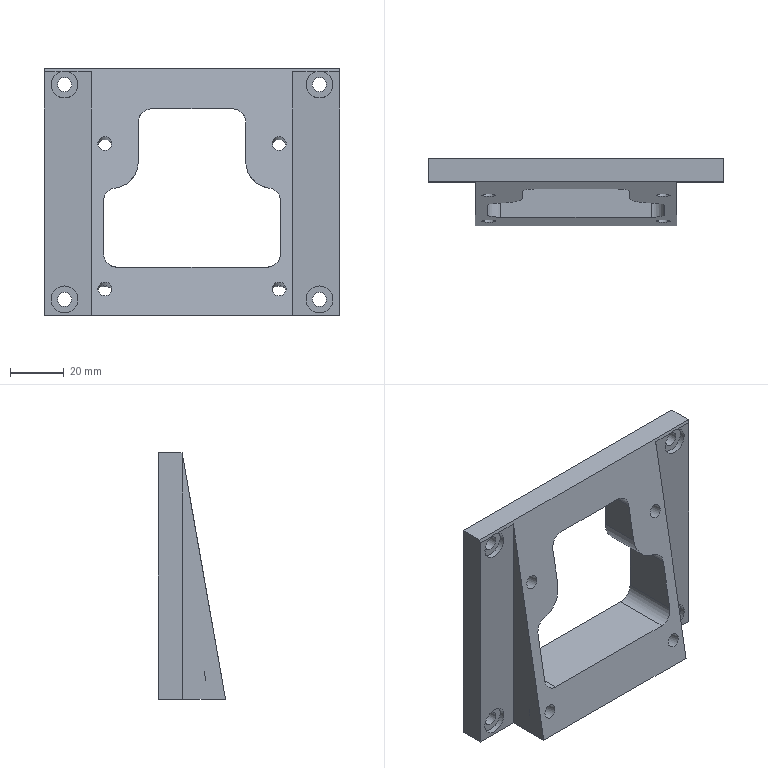Part | 1 solid | 48 faces | box 110 x 25 x 92 mm | volume 85640 mm3 | plane 24 | cylinder 24 | commonest cylinder face diameters 10 x14 5.2 x4 5.3 x4 20 x2
STEP:
#1=CARTESIAN_POINT('',(-37.5,3.5,44.741));
#2=VERTEX_POINT('',#1);
#3=CARTESIAN_POINT('',(-37.5,-12.5,-46.));
#4=VERTEX_POINT('',#3);
#5=CARTESIAN_POINT('',(-37.5,3.5,44.741));
#6=DIRECTION('',(0.,-0.1736,-0.9848));
#7=VECTOR('',#6,1000.);
#8=LINE('',#5,#7);
#9=EDGE_CURVE('',#2,#4,#8,.T.);
#10=ORIENTED_EDGE('',*,*,#9,.F.);
#11=CARTESIAN_POINT('',(-37.5,3.5,-46.));
#12=VERTEX_POINT('',#11);
#13=CARTESIAN_POINT('',(-37.5,3.5,-46.));
#14=DIRECTION('',(0.,0.,1.));
#15=VECTOR('',#14,1000.);
#16=LINE('',#13,#15);
#17=EDGE_CURVE('',#12,#2,#16,.T.);
#18=ORIENTED_EDGE('',*,*,#17,.F.);
#19=CARTESIAN_POINT('',(-37.5,-12.5,-46.));
#20=DIRECTION('',(0.,1.,0.));
#21=VECTOR('',#20,1000.);
#22=LINE('',#19,#21);
#23=EDGE_CURVE('',#4,#12,#22,.T.);
#24=ORIENTED_EDGE('',*,*,#23,.F.);
#25=EDGE_LOOP('',(#10,#18,#24));
#26=FACE_BOUND('',#25,.T.);
#27=CARTESIAN_POINT('',(-37.5,3.5,-46.));
#28=DIRECTION('',(1.,0.,0.));
#29=DIRECTION('',(0.,-1.,0.));
#30=AXIS2_PLACEMENT_3D('',#27,#28,#29);
#31=PLANE('',#30);
#32=ADVANCED_FACE('',(#26),#31,.F.);
#33=CARTESIAN_POINT('',(50.15,12.5,-40.));
#34=VERTEX_POINT('',#33);
#35=CARTESIAN_POINT('',(47.5,12.5,-40.));
#36=DIRECTION('',(0.,-1.,0.));
#37=DIRECTION('',(1.,0.,0.));
#38=AXIS2_PLACEMENT_3D('',#35,#36,#37);
#39=CIRCLE('',#38,2.65);
#40=EDGE_CURVE('',#34,#34,#39,.T.);
#41=ORIENTED_EDGE('',*,*,#40,.F.);
#42=EDGE_LOOP('',(#41));
#43=FACE_BOUND('',#42,.T.);
#44=CARTESIAN_POINT('',(44.85,5.5,-40.));
#45=VERTEX_POINT('',#44);
#46=CARTESIAN_POINT('',(47.5,5.5,-40.));
#47=DIRECTION('',(0.,1.,0.));
#48=DIRECTION('',(-1.,0.,0.));
#49=AXIS2_PLACEMENT_3D('',#46,#47,#48);
#50=CIRCLE('',#49,2.65);
#51=EDGE_CURVE('',#45,#45,#50,.T.);
#52=ORIENTED_EDGE('',*,*,#51,.F.);
#53=EDGE_LOOP('',(#52));
#54=FACE_BOUND('',#53,.T.);
#55=CARTESIAN_POINT('',(47.5,-16.47,-40.));
#56=DIRECTION('',(0.,-1.,0.));
#57=DIRECTION('',(-1.,0.,0.));
#58=AXIS2_PLACEMENT_3D('',#55,#56,#57);
#59=CYLINDRICAL_SURFACE('',#58,2.65);
#60=ADVANCED_FACE('',(#43,#54),#59,.F.);
#61=CARTESIAN_POINT('',(50.15,12.5,40.));
#62=VERTEX_POINT('',#61);
#63=CARTESIAN_POINT('',(47.5,12.5,40.));
#64=DIRECTION('',(0.,-1.,0.));
#65=DIRECTION('',(1.,0.,0.));
#66=AXIS2_PLACEMENT_3D('',#63,#64,#65);
#67=CIRCLE('',#66,2.65);
#68=EDGE_CURVE('',#62,#62,#67,.T.);
#69=ORIENTED_EDGE('',*,*,#68,.F.);
#70=EDGE_LOOP('',(#69));
#71=FACE_BOUND('',#70,.T.);
#72=CARTESIAN_POINT('',(44.85,5.5,40.));
#73=VERTEX_POINT('',#72);
#74=CARTESIAN_POINT('',(47.5,5.5,40.));
#75=DIRECTION('',(0.,1.,0.));
#76=DIRECTION('',(-1.,0.,0.));
#77=AXIS2_PLACEMENT_3D('',#74,#75,#76);
#78=CIRCLE('',#77,2.65);
#79=EDGE_CURVE('',#73,#73,#78,.T.);
#80=ORIENTED_EDGE('',*,*,#79,.F.);
#81=EDGE_LOOP('',(#80));
#82=FACE_BOUND('',#81,.T.);
#83=CARTESIAN_POINT('',(47.5,-16.47,40.));
#84=DIRECTION('',(0.,-1.,0.));
#85=DIRECTION('',(-1.,0.,0.));
#86=AXIS2_PLACEMENT_3D('',#83,#84,#85);
#87=CYLINDRICAL_SURFACE('',#86,2.65);
#88=ADVANCED_FACE('',(#71,#82),#87,.F.);
#89=CARTESIAN_POINT('',(-50.15,12.5,-40.));
#90=VERTEX_POINT('',#89);
#91=CARTESIAN_POINT('',(-47.5,12.5,-40.));
#92=DIRECTION('',(0.,1.,0.));
#93=DIRECTION('',(-1.,0.,0.));
#94=AXIS2_PLACEMENT_3D('',#91,#92,#93);
#95=CIRCLE('',#94,2.65);
#96=EDGE_CURVE('',#90,#90,#95,.T.);
#97=ORIENTED_EDGE('',*,*,#96,.T.);
#98=EDGE_LOOP('',(#97));
#99=FACE_BOUND('',#98,.T.);
#100=CARTESIAN_POINT('',(-44.85,5.5,-40.));
#101=VERTEX_POINT('',#100);
#102=CARTESIAN_POINT('',(-47.5,5.5,-40.));
#103=DIRECTION('',(0.,-1.,0.));
#104=DIRECTION('',(1.,0.,0.));
#105=AXIS2_PLACEMENT_3D('',#102,#103,#104);
#106=CIRCLE('',#105,2.65);
#107=EDGE_CURVE('',#101,#101,#106,.T.);
#108=ORIENTED_EDGE('',*,*,#107,.T.);
#109=EDGE_LOOP('',(#108));
#110=FACE_BOUND('',#109,.T.);
#111=CARTESIAN_POINT('',(-47.5,-16.47,-40.));
#112=DIRECTION('',(0.,1.,0.));
#113=DIRECTION('',(1.,0.,0.));
#114=AXIS2_PLACEMENT_3D('',#111,#112,#113);
#115=CYLINDRICAL_SURFACE('',#114,2.65);
#116=ADVANCED_FACE('',(#99,#110),#115,.F.);
#117=CARTESIAN_POINT('',(-50.15,12.5,40.));
#118=VERTEX_POINT('',#117);
#119=CARTESIAN_POINT('',(-47.5,12.5,40.));
#120=DIRECTION('',(0.,1.,0.));
#121=DIRECTION('',(-1.,0.,0.));
#122=AXIS2_PLACEMENT_3D('',#119,#120,#121);
#123=CIRCLE('',#122,2.65);
#124=EDGE_CURVE('',#118,#118,#123,.T.);
#125=ORIENTED_EDGE('',*,*,#124,.T.);
#126=EDGE_LOOP('',(#125));
#127=FACE_BOUND('',#126,.T.);
#128=CARTESIAN_POINT('',(-44.85,5.5,40.));
#129=VERTEX_POINT('',#128);
#130=CARTESIAN_POINT('',(-47.5,5.5,40.));
#131=DIRECTION('',(0.,-1.,0.));
#132=DIRECTION('',(1.,0.,0.));
#133=AXIS2_PLACEMENT_3D('',#130,#131,#132);
#134=CIRCLE('',#133,2.65);
#135=EDGE_CURVE('',#129,#129,#134,.T.);
#136=ORIENTED_EDGE('',*,*,#135,.T.);
#137=EDGE_LOOP('',(#136));
#138=FACE_BOUND('',#137,.T.);
#139=CARTESIAN_POINT('',(-47.5,-16.452,40.));
#140=DIRECTION('',(0.,1.,0.));
#141=DIRECTION('',(1.,0.,0.));
#142=AXIS2_PLACEMENT_3D('',#139,#140,#141);
#143=CYLINDRICAL_SURFACE('',#142,2.65);
#144=ADVANCED_FACE('',(#127,#138),#143,.F.);
#145=CARTESIAN_POINT('',(-47.5,5.5,45.));
#146=VERTEX_POINT('',#145);
#147=CARTESIAN_POINT('',(-47.5,5.5,40.));
#148=DIRECTION('',(0.,-1.,0.));
#149=DIRECTION('',(0.,0.,1.));
#150=AXIS2_PLACEMENT_3D('',#147,#148,#149);
#151=CIRCLE('',#150,5.);
#152=EDGE_CURVE('',#146,#146,#151,.T.);
#153=ORIENTED_EDGE('',*,*,#152,.F.);
#154=EDGE_LOOP('',(#153));
#155=FACE_BOUND('',#154,.T.);
#156=CARTESIAN_POINT('',(-45.91,3.5,44.741));
#157=VERTEX_POINT('',#156);
#158=CARTESIAN_POINT('',(-49.09,3.5,44.741));
#159=VERTEX_POINT('',#158);
#160=CARTESIAN_POINT('',(-47.5,3.5,40.));
#161=DIRECTION('',(0.,1.,0.));
#162=DIRECTION('',(0.318,0.,0.9481));
#163=AXIS2_PLACEMENT_3D('',#160,#161,#162);
#164=CIRCLE('',#163,5.);
#165=EDGE_CURVE('',#157,#159,#164,.T.);
#166=ORIENTED_EDGE('',*,*,#165,.F.);
#167=CARTESIAN_POINT('',(-47.5,2.664,40.));
#168=DIRECTION('',(0.,0.9848,-0.1736));
#169=DIRECTION('',(0.,0.1736,0.9848));
#170=AXIS2_PLACEMENT_3D('',#167,#168,#169);
#171=ELLIPSE('',#170,5.077,5.);
#172=EDGE_CURVE('',#159,#157,#171,.T.);
#173=ORIENTED_EDGE('',*,*,#172,.F.);
#174=EDGE_LOOP('',(#166,#173));
#175=FACE_BOUND('',#174,.T.);
#176=CARTESIAN_POINT('',(-47.5,5.5,40.));
#177=DIRECTION('',(0.,1.,0.));
#178=DIRECTION('',(0.,0.,1.));
#179=AXIS2_PLACEMENT_3D('',#176,#177,#178);
#180=CYLINDRICAL_SURFACE('',#179,5.);
#181=ADVANCED_FACE('',(#155,#175),#180,.F.);
#182=CARTESIAN_POINT('',(-47.5,5.5,-35.));
#183=VERTEX_POINT('',#182);
#184=CARTESIAN_POINT('',(-47.5,5.5,-40.));
#185=DIRECTION('',(0.,-1.,0.));
#186=DIRECTION('',(0.,0.,1.));
#187=AXIS2_PLACEMENT_3D('',#184,#185,#186);
#188=CIRCLE('',#187,5.);
#189=EDGE_CURVE('',#183,#183,#188,.T.);
#190=ORIENTED_EDGE('',*,*,#189,.F.);
#191=EDGE_LOOP('',(#190));
#192=FACE_BOUND('',#191,.T.);
#193=CARTESIAN_POINT('',(-47.5,3.5,-45.));
#194=VERTEX_POINT('',#193);
#195=CARTESIAN_POINT('',(-47.5,3.5,-40.));
#196=DIRECTION('',(0.,1.,0.));
#197=DIRECTION('',(0.,0.,-1.));
#198=AXIS2_PLACEMENT_3D('',#195,#196,#197);
#199=CIRCLE('',#198,5.);
#200=EDGE_CURVE('',#194,#194,#199,.T.);
#201=ORIENTED_EDGE('',*,*,#200,.F.);
#202=EDGE_LOOP('',(#201));
#203=FACE_BOUND('',#202,.T.);
#204=CARTESIAN_POINT('',(-47.5,5.5,-40.));
#205=DIRECTION('',(0.,1.,0.));
#206=DIRECTION('',(0.,0.,1.));
#207=AXIS2_PLACEMENT_3D('',#204,#205,#206);
#208=CYLINDRICAL_SURFACE('',#207,5.);
#209=ADVANCED_FACE('',(#192,#203),#208,.F.);
#210=CARTESIAN_POINT('',(47.5,5.5,-35.));
#211=VERTEX_POINT('',#210);
#212=CARTESIAN_POINT('',(47.5,5.5,-40.));
#213=DIRECTION('',(0.,-1.,0.));
#214=DIRECTION('',(0.,0.,1.));
#215=AXIS2_PLACEMENT_3D('',#212,#213,#214);
#216=CIRCLE('',#215,5.);
#217=EDGE_CURVE('',#211,#211,#216,.T.);
#218=ORIENTED_EDGE('',*,*,#217,.F.);
#219=EDGE_LOOP('',(#218));
#220=FACE_BOUND('',#219,.T.);
#221=CARTESIAN_POINT('',(47.5,3.5,-35.));
#222=VERTEX_POINT('',#221);
#223=CARTESIAN_POINT('',(47.5,3.5,-40.));
#224=DIRECTION('',(0.,1.,0.));
#225=DIRECTION('',(0.,0.,1.));
#226=AXIS2_PLACEMENT_3D('',#223,#224,#225);
#227=CIRCLE('',#226,5.);
#228=EDGE_CURVE('',#222,#222,#227,.T.);
#229=ORIENTED_EDGE('',*,*,#228,.F.);
#230=EDGE_LOOP('',(#229));
#231=FACE_BOUND('',#230,.T.);
#232=CARTESIAN_POINT('',(47.5,5.5,-40.));
#233=DIRECTION('',(0.,1.,0.));
#234=DIRECTION('',(0.,0.,1.));
#235=AXIS2_PLACEMENT_3D('',#232,#233,#234);
#236=CYLINDRICAL_SURFACE('',#235,5.);
#237=ADVANCED_FACE('',(#220,#231),#236,.F.);
#238=ORIENTED_EDGE('',*,*,#135,.F.);
#239=EDGE_LOOP('',(#238));
#240=FACE_BOUND('',#239,.T.);
#241=ORIENTED_EDGE('',*,*,#152,.T.);
#242=EDGE_LOOP('',(#241));
#243=FACE_BOUND('',#242,.T.);
#244=CARTESIAN_POINT('',(0.,5.5,0.));
#245=DIRECTION('',(0.,1.,0.));
#246=DIRECTION('',(0.,0.,1.));
#247=AXIS2_PLACEMENT_3D('',#244,#245,#246);
#248=PLANE('',#247);
#249=ADVANCED_FACE('',(#240,#243),#248,.F.);
#250=ORIENTED_EDGE('',*,*,#107,.F.);
#251=EDGE_LOOP('',(#250));
#252=FACE_BOUND('',#251,.T.);
#253=ORIENTED_EDGE('',*,*,#189,.T.);
#254=EDGE_LOOP('',(#253));
#255=FACE_BOUND('',#254,.T.);
#256=CARTESIAN_POINT('',(0.,5.5,0.));
#257=DIRECTION('',(0.,1.,0.));
#258=DIRECTION('',(0.,0.,1.));
#259=AXIS2_PLACEMENT_3D('',#256,#257,#258);
#260=PLANE('',#259);
#261=ADVANCED_FACE('',(#252,#255),#260,.F.);
#262=ORIENTED_EDGE('',*,*,#79,.T.);
#263=EDGE_LOOP('',(#262));
#264=FACE_BOUND('',#263,.T.);
#265=CARTESIAN_POINT('',(47.5,5.5,45.));
#266=VERTEX_POINT('',#265);
#267=CARTESIAN_POINT('',(47.5,5.5,40.));
#268=DIRECTION('',(0.,-1.,0.));
#269=DIRECTION('',(0.,0.,1.));
#270=AXIS2_PLACEMENT_3D('',#267,#268,#269);
#271=CIRCLE('',#270,5.);
#272=EDGE_CURVE('',#266,#266,#271,.T.);
#273=ORIENTED_EDGE('',*,*,#272,.T.);
#274=EDGE_LOOP('',(#273));
#275=FACE_BOUND('',#274,.T.);
#276=CARTESIAN_POINT('',(0.,5.5,0.));
#277=DIRECTION('',(0.,1.,0.));
#278=DIRECTION('',(0.,0.,1.));
#279=AXIS2_PLACEMENT_3D('',#276,#277,#278);
#280=PLANE('',#279);
#281=ADVANCED_FACE('',(#264,#275),#280,.F.);
#282=ORIENTED_EDGE('',*,*,#51,.T.);
#283=EDGE_LOOP('',(#282));
#284=FACE_BOUND('',#283,.T.);
#285=ORIENTED_EDGE('',*,*,#217,.T.);
#286=EDGE_LOOP('',(#285));
#287=FACE_BOUND('',#286,.T.);
#288=CARTESIAN_POINT('',(0.,5.5,0.));
#289=DIRECTION('',(0.,1.,0.));
#290=DIRECTION('',(0.,0.,1.));
#291=AXIS2_PLACEMENT_3D('',#288,#289,#290);
#292=PLANE('',#291);
#293=ADVANCED_FACE('',(#284,#287),#292,.F.);
#294=CARTESIAN_POINT('',(45.91,3.5,44.741));
#295=VERTEX_POINT('',#294);
#296=CARTESIAN_POINT('',(49.09,3.5,44.741));
#297=VERTEX_POINT('',#296);
#298=CARTESIAN_POINT('',(47.5,2.664,40.));
#299=DIRECTION('',(0.,0.9848,-0.1736));
#300=DIRECTION('',(0.,0.1736,0.9848));
#301=AXIS2_PLACEMENT_3D('',#298,#299,#300);
#302=ELLIPSE('',#301,5.077,5.);
#303=EDGE_CURVE('',#295,#297,#302,.T.);
#304=ORIENTED_EDGE('',*,*,#303,.F.);
#305=CARTESIAN_POINT('',(47.5,3.5,40.));
#306=DIRECTION('',(0.,1.,0.));
#307=DIRECTION('',(0.,0.,1.));
#308=AXIS2_PLACEMENT_3D('',#305,#306,#307);
#309=CIRCLE('',#308,5.);
#310=EDGE_CURVE('',#297,#295,#309,.T.);
#311=ORIENTED_EDGE('',*,*,#310,.F.);
#312=EDGE_LOOP('',(#304,#311));
#313=FACE_BOUND('',#312,.T.);
#314=ORIENTED_EDGE('',*,*,#272,.F.);
#315=EDGE_LOOP('',(#314));
#316=FACE_BOUND('',#315,.T.);
#317=CARTESIAN_POINT('',(47.5,5.5,40.));
#318=DIRECTION('',(0.,1.,0.));
#319=DIRECTION('',(0.,0.,1.));
#320=AXIS2_PLACEMENT_3D('',#317,#318,#319);
#321=CYLINDRICAL_SURFACE('',#320,5.);
#322=ADVANCED_FACE('',(#313,#316),#321,.F.);
#323=CARTESIAN_POINT('',(-55.,3.722,46.));
#324=VERTEX_POINT('',#323);
#325=CARTESIAN_POINT('',(55.,3.722,46.));
#326=VERTEX_POINT('',#325);
#327=CARTESIAN_POINT('',(-55.,3.722,46.));
#328=DIRECTION('',(1.,0.,0.));
#329=VECTOR('',#328,1000.);
#330=LINE('',#327,#329);
#331=EDGE_CURVE('',#324,#326,#330,.T.);
#332=ORIENTED_EDGE('',*,*,#331,.T.);
#333=CARTESIAN_POINT('',(55.,12.5,46.));
#334=VERTEX_POINT('',#333);
#335=CARTESIAN_POINT('',(55.,3.722,46.));
#336=DIRECTION('',(0.,1.,0.));
#337=VECTOR('',#336,1000.);
#338=LINE('',#335,#337);
#339=EDGE_CURVE('',#326,#334,#338,.T.);
#340=ORIENTED_EDGE('',*,*,#339,.T.);
#341=CARTESIAN_POINT('',(-55.,12.5,46.));
#342=VERTEX_POINT('',#341);
#343=CARTESIAN_POINT('',(-55.,12.5,46.));
#344=DIRECTION('',(1.,0.,0.));
#345=VECTOR('',#344,1000.);
#346=LINE('',#343,#345);
#347=EDGE_CURVE('',#342,#334,#346,.T.);
#348=ORIENTED_EDGE('',*,*,#347,.F.);
#349=CARTESIAN_POINT('',(-55.,3.722,46.));
#350=DIRECTION('',(0.,1.,0.));
#351=VECTOR('',#350,1000.);
#352=LINE('',#349,#351);
#353=EDGE_CURVE('',#324,#342,#352,.T.);
#354=ORIENTED_EDGE('',*,*,#353,.F.);
#355=EDGE_LOOP('',(#332,#340,#348,#354));
#356=FACE_BOUND('',#355,.T.);
#357=CARTESIAN_POINT('',(-55.,-12.5,46.));
#358=DIRECTION('',(0.,0.,1.));
#359=DIRECTION('',(1.,0.,0.));
#360=AXIS2_PLACEMENT_3D('',#357,#358,#359);
#361=PLANE('',#360);
#362=ADVANCED_FACE('',(#356),#361,.T.);
#363=CARTESIAN_POINT('',(55.,3.5,-46.));
#364=VERTEX_POINT('',#363);
#365=CARTESIAN_POINT('',(55.,12.5,-46.));
#366=VERTEX_POINT('',#365);
#367=CARTESIAN_POINT('',(55.,3.5,-46.));
#368=DIRECTION('',(0.,1.,0.));
#369=VECTOR('',#368,1000.);
#370=LINE('',#367,#369);
#371=EDGE_CURVE('',#364,#366,#370,.T.);
#372=ORIENTED_EDGE('',*,*,#371,.T.);
#373=CARTESIAN_POINT('',(55.,12.5,46.));
#374=DIRECTION('',(0.,0.,-1.));
#375=VECTOR('',#374,1000.);
#376=LINE('',#373,#375);
#377=EDGE_CURVE('',#334,#366,#376,.T.);
#378=ORIENTED_EDGE('',*,*,#377,.F.);
#379=ORIENTED_EDGE('',*,*,#339,.F.);
#380=CARTESIAN_POINT('',(55.,3.5,44.741));
#381=VERTEX_POINT('',#380);
#382=CARTESIAN_POINT('',(55.,3.722,46.));
#383=DIRECTION('',(0.,-0.1736,-0.9848));
#384=VECTOR('',#383,1000.);
#385=LINE('',#382,#384);
#386=EDGE_CURVE('',#326,#381,#385,.T.);
#387=ORIENTED_EDGE('',*,*,#386,.T.);
#388=CARTESIAN_POINT('',(55.,3.5,46.));
#389=DIRECTION('',(0.,0.,-1.));
#390=VECTOR('',#389,1000.);
#391=LINE('',#388,#390);
#392=EDGE_CURVE('',#381,#364,#391,.T.);
#393=ORIENTED_EDGE('',*,*,#392,.T.);
#394=EDGE_LOOP('',(#372,#378,#379,#387,#393));
#395=FACE_BOUND('',#394,.T.);
#396=CARTESIAN_POINT('',(55.,-12.5,46.));
#397=DIRECTION('',(1.,0.,0.));
#398=DIRECTION('',(0.,0.,-1.));
#399=AXIS2_PLACEMENT_3D('',#396,#397,#398);
#400=PLANE('',#399);
#401=ADVANCED_FACE('',(#395),#400,.T.);
#402=ORIENTED_EDGE('',*,*,#228,.T.);
#403=EDGE_LOOP('',(#402));
#404=FACE_BOUND('',#403,.T.);
#405=CARTESIAN_POINT('',(-55.,3.5,44.741));
#406=DIRECTION('',(-1.,0.,0.));
#407=VECTOR('',#406,1000.);
#408=LINE('',#405,#407);
#409=EDGE_CURVE('',#381,#297,#408,.T.);
#410=ORIENTED_EDGE('',*,*,#409,.T.);
#411=ORIENTED_EDGE('',*,*,#310,.T.);
#412=CARTESIAN_POINT('',(37.5,3.5,44.741));
#413=VERTEX_POINT('',#412);
#414=CARTESIAN_POINT('',(-55.,3.5,44.741));
#415=DIRECTION('',(-1.,0.,0.));
#416=VECTOR('',#415,1000.);
#417=LINE('',#414,#416);
#418=EDGE_CURVE('',#295,#413,#417,.T.);
#419=ORIENTED_EDGE('',*,*,#418,.T.);
#420=CARTESIAN_POINT('',(37.5,3.5,-46.));
#421=VERTEX_POINT('',#420);
#422=CARTESIAN_POINT('',(37.5,3.5,-46.));
#423=DIRECTION('',(0.,0.,1.));
#424=VECTOR('',#423,1000.);
#425=LINE('',#422,#424);
#426=EDGE_CURVE('',#421,#413,#425,.T.);
#427=ORIENTED_EDGE('',*,*,#426,.F.);
#428=CARTESIAN_POINT('',(55.,3.5,-46.));
#429=DIRECTION('',(-1.,0.,0.));
#430=VECTOR('',#429,1000.);
#431=LINE('',#428,#430);
#432=EDGE_CURVE('',#364,#421,#431,.T.);
#433=ORIENTED_EDGE('',*,*,#432,.F.);
#434=ORIENTED_EDGE('',*,*,#392,.F.);
#435=EDGE_LOOP('',(#410,#411,#419,#427,#433,#434));
#436=FACE_BOUND('',#435,.T.);
#437=CARTESIAN_POINT('',(-55.,3.5,-46.));
#438=DIRECTION('',(0.,1.,0.));
#439=DIRECTION('',(1.,0.,0.));
#440=AXIS2_PLACEMENT_3D('',#437,#438,#439);
#441=PLANE('',#440);
#442=ADVANCED_FACE('',(#404,#436),#441,.F.);
#443=CARTESIAN_POINT('',(37.5,-12.5,-46.));
#444=VERTEX_POINT('',#443);
#445=CARTESIAN_POINT('',(-37.5,-12.5,-46.));
#446=DIRECTION('',(1.,0.,0.));
#447=VECTOR('',#446,1000.);
#448=LINE('',#445,#447);
#449=EDGE_CURVE('',#4,#444,#448,.T.);
#450=ORIENTED_EDGE('',*,*,#449,.F.);
#451=ORIENTED_EDGE('',*,*,#23,.T.);
#452=CARTESIAN_POINT('',(-55.,3.5,-46.));
#453=VERTEX_POINT('',#452);
#454=CARTESIAN_POINT('',(-55.,3.5,-46.));
#455=DIRECTION('',(1.,0.,0.));
#456=VECTOR('',#455,1000.);
#457=LINE('',#454,#456);
#458=EDGE_CURVE('',#453,#12,#457,.T.);
#459=ORIENTED_EDGE('',*,*,#458,.F.);
#460=CARTESIAN_POINT('',(-55.,12.5,-46.));
#461=VERTEX_POINT('',#460);
#462=CARTESIAN_POINT('',(-55.,3.5,-46.));
#463=DIRECTION('',(0.,1.,0.));
#464=VECTOR('',#463,1000.);
#465=LINE('',#462,#464);
#466=EDGE_CURVE('',#453,#461,#465,.T.);
#467=ORIENTED_EDGE('',*,*,#466,.T.);
#468=CARTESIAN_POINT('',(55.,12.5,-46.));
#469=DIRECTION('',(-1.,0.,0.));
#470=VECTOR('',#469,1000.);
#471=LINE('',#468,#470);
#472=EDGE_CURVE('',#366,#461,#471,.T.);
#473=ORIENTED_EDGE('',*,*,#472,.F.);
#474=ORIENTED_EDGE('',*,*,#371,.F.);
#475=ORIENTED_EDGE('',*,*,#432,.T.);
#476=CARTESIAN_POINT('',(37.5,-12.5,-46.));
#477=DIRECTION('',(0.,1.,0.));
#478=VECTOR('',#477,1000.);
#479=LINE('',#476,#478);
#480=EDGE_CURVE('',#444,#421,#479,.T.);
#481=ORIENTED_EDGE('',*,*,#480,.F.);
#482=EDGE_LOOP('',(#450,#451,#459,#467,#473,#474,#475,#481));
#483=FACE_BOUND('',#482,.T.);
#484=CARTESIAN_POINT('',(55.,-12.5,-46.));
#485=DIRECTION('',(0.,0.,-1.));
#486=DIRECTION('',(-1.,0.,0.));
#487=AXIS2_PLACEMENT_3D('',#484,#485,#486);
#488=PLANE('',#487);
#489=ADVANCED_FACE('',(#483),#488,.T.);
#490=ORIENTED_EDGE('',*,*,#426,.T.);
#491=CARTESIAN_POINT('',(37.5,3.5,44.741));
#492=DIRECTION('',(0.,-0.1736,-0.9848));
#493=VECTOR('',#492,1000.);
#494=LINE('',#491,#493);
#495=EDGE_CURVE('',#413,#444,#494,.T.);
#496=ORIENTED_EDGE('',*,*,#495,.T.);
#497=ORIENTED_EDGE('',*,*,#480,.T.);
#498=EDGE_LOOP('',(#490,#496,#497));
#499=FACE_BOUND('',#498,.T.);
#500=CARTESIAN_POINT('',(37.5,-12.5,-46.));
#501=DIRECTION('',(-1.,0.,0.));
#502=DIRECTION('',(0.,1.,0.));
#503=AXIS2_PLACEMENT_3D('',#500,#501,#502);
#504=PLANE('',#503);
#505=ADVANCED_FACE('',(#499),#504,.F.);
#506=CARTESIAN_POINT('',(-20.,0.1955,26.));
#507=VERTEX_POINT('',#506);
#508=CARTESIAN_POINT('',(-15.,1.077,31.));
#509=VERTEX_POINT('',#508);
#510=CARTESIAN_POINT('',(-15.,0.1955,26.));
#511=DIRECTION('',(0.,0.9848,-0.1736));
#512=DIRECTION('',(0.,-0.1736,-0.9848));
#513=AXIS2_PLACEMENT_3D('',#510,#511,#512);
#514=ELLIPSE('',#513,5.077,5.);
#515=EDGE_CURVE('',#507,#509,#514,.T.);
#516=ORIENTED_EDGE('',*,*,#515,.F.);
#517=CARTESIAN_POINT('',(-20.,12.5,26.));
#518=VERTEX_POINT('',#517);
#519=CARTESIAN_POINT('',(-20.,12.5,26.));
#520=DIRECTION('',(0.,-1.,0.));
#521=VECTOR('',#520,1000.);
#522=LINE('',#519,#521);
#523=EDGE_CURVE('',#518,#507,#522,.T.);
#524=ORIENTED_EDGE('',*,*,#523,.F.);
#525=CARTESIAN_POINT('',(-15.,12.5,31.));
#526=VERTEX_POINT('',#525);
#527=CARTESIAN_POINT('',(-15.,12.5,26.));
#528=DIRECTION('',(0.,-1.,0.));
#529=DIRECTION('',(0.,0.,1.));
#530=AXIS2_PLACEMENT_3D('',#527,#528,#529);
#531=CIRCLE('',#530,5.);
#532=EDGE_CURVE('',#526,#518,#531,.T.);
#533=ORIENTED_EDGE('',*,*,#532,.F.);
#534=CARTESIAN_POINT('',(-15.,12.5,31.));
#535=DIRECTION('',(0.,-1.,0.));
#536=VECTOR('',#535,1000.);
#537=LINE('',#534,#536);
#538=EDGE_CURVE('',#526,#509,#537,.T.);
#539=ORIENTED_EDGE('',*,*,#538,.T.);
#540=EDGE_LOOP('',(#516,#524,#533,#539));
#541=FACE_BOUND('',#540,.T.);
#542=CARTESIAN_POINT('',(-15.,49.09,26.));
#543=DIRECTION('',(0.,-1.,0.));
#544=DIRECTION('',(0.,0.,1.));
#545=AXIS2_PLACEMENT_3D('',#542,#543,#544);
#546=CYLINDRICAL_SURFACE('',#545,5.);
#547=ADVANCED_FACE('',(#541),#546,.F.);
#548=CARTESIAN_POINT('',(15.,1.077,31.));
#549=VERTEX_POINT('',#548);
#550=CARTESIAN_POINT('',(-15.,1.077,31.));
#551=DIRECTION('',(1.,0.,0.));
#552=VECTOR('',#551,1000.);
#553=LINE('',#550,#552);
#554=EDGE_CURVE('',#509,#549,#553,.T.);
#555=ORIENTED_EDGE('',*,*,#554,.F.);
#556=ORIENTED_EDGE('',*,*,#538,.F.);
#557=CARTESIAN_POINT('',(15.,12.5,31.));
#558=VERTEX_POINT('',#557);
#559=CARTESIAN_POINT('',(-15.,12.5,31.));
#560=DIRECTION('',(1.,0.,0.));
#561=VECTOR('',#560,1000.);
#562=LINE('',#559,#561);
#563=EDGE_CURVE('',#526,#558,#562,.T.);
#564=ORIENTED_EDGE('',*,*,#563,.T.);
#565=CARTESIAN_POINT('',(15.,12.5,31.));
#566=DIRECTION('',(0.,-1.,0.));
#567=VECTOR('',#566,1000.);
#568=LINE('',#565,#567);
#569=EDGE_CURVE('',#558,#549,#568,.T.);
#570=ORIENTED_EDGE('',*,*,#569,.T.);
#571=EDGE_LOOP('',(#555,#556,#564,#570));
#572=FACE_BOUND('',#571,.T.);
#573=CARTESIAN_POINT('',(-20.,12.5,31.));
#574=DIRECTION('',(0.,0.,1.));
#575=DIRECTION('',(1.,0.,0.));
#576=AXIS2_PLACEMENT_3D('',#573,#574,#575);
#577=PLANE('',#576);
#578=ADVANCED_FACE('',(#572),#577,.F.);
#579=CARTESIAN_POINT('',(20.,0.1955,26.));
#580=VERTEX_POINT('',#579);
#581=CARTESIAN_POINT('',(15.,0.1955,26.));
#582=DIRECTION('',(0.,0.9848,-0.1736));
#583=DIRECTION('',(0.,-0.1736,-0.9848));
#584=AXIS2_PLACEMENT_3D('',#581,#582,#583);
#585=ELLIPSE('',#584,5.077,5.);
#586=EDGE_CURVE('',#549,#580,#585,.T.);
#587=ORIENTED_EDGE('',*,*,#586,.F.);
#588=ORIENTED_EDGE('',*,*,#569,.F.);
#589=CARTESIAN_POINT('',(20.,12.5,26.));
#590=VERTEX_POINT('',#589);
#591=CARTESIAN_POINT('',(15.,12.5,26.));
#592=DIRECTION('',(0.,-1.,0.));
#593=DIRECTION('',(1.,0.,0.));
#594=AXIS2_PLACEMENT_3D('',#591,#592,#593);
#595=CIRCLE('',#594,5.);
#596=EDGE_CURVE('',#590,#558,#595,.T.);
#597=ORIENTED_EDGE('',*,*,#596,.F.);
#598=CARTESIAN_POINT('',(20.,12.5,26.));
#599=DIRECTION('',(0.,-1.,0.));
#600=VECTOR('',#599,1000.);
#601=LINE('',#598,#600);
#602=EDGE_CURVE('',#590,#580,#601,.T.);
#603=ORIENTED_EDGE('',*,*,#602,.T.);
#604=EDGE_LOOP('',(#587,#588,#597,#603));
#605=FACE_BOUND('',#604,.T.);
#606=CARTESIAN_POINT('',(15.,49.09,26.));
#607=DIRECTION('',(0.,-1.,0.));
#608=DIRECTION('',(1.,0.,0.));
#609=AXIS2_PLACEMENT_3D('',#606,#607,#608);
#610=CYLINDRICAL_SURFACE('',#609,5.);
#611=ADVANCED_FACE('',(#605),#610,.F.);
#612=CARTESIAN_POINT('',(20.,-2.385,11.366));
#613=VERTEX_POINT('',#612);
#614=CARTESIAN_POINT('',(20.,12.5,11.366));
#615=VERTEX_POINT('',#614);
#616=CARTESIAN_POINT('',(20.,49.09,11.366));
#617=DIRECTION('',(0.,1.,0.));
#618=VECTOR('',#617,1000.);
#619=LINE('',#616,#618);
#620=EDGE_CURVE('',#613,#615,#619,.T.);
#621=ORIENTED_EDGE('',*,*,#620,.F.);
#622=CARTESIAN_POINT('',(20.,0.1955,26.));
#623=DIRECTION('',(0.,-0.1736,-0.9848));
#624=VECTOR('',#623,1000.);
#625=LINE('',#622,#624);
#626=EDGE_CURVE('',#580,#613,#625,.T.);
#627=ORIENTED_EDGE('',*,*,#626,.F.);
#628=ORIENTED_EDGE('',*,*,#602,.F.);
#629=CARTESIAN_POINT('',(20.,12.5,26.));
#630=DIRECTION('',(0.,0.,-1.));
#631=VECTOR('',#630,1000.);
#632=LINE('',#629,#631);
#633=EDGE_CURVE('',#590,#615,#632,.T.);
#634=ORIENTED_EDGE('',*,*,#633,.T.);
#635=EDGE_LOOP('',(#621,#627,#628,#634));
#636=FACE_BOUND('',#635,.T.);
#637=CARTESIAN_POINT('',(20.,12.5,31.));
#638=DIRECTION('',(1.,0.,0.));
#639=DIRECTION('',(0.,0.,-1.));
#640=AXIS2_PLACEMENT_3D('',#637,#638,#639);
#641=PLANE('',#640);
#642=ADVANCED_FACE('',(#636),#641,.F.);
#643=CARTESIAN_POINT('',(28.667,-4.132,1.455));
#644=VERTEX_POINT('',#643);
#645=CARTESIAN_POINT('',(28.667,12.5,1.455));
#646=VERTEX_POINT('',#645);
#647=CARTESIAN_POINT('',(28.667,-4.132,1.455));
#648=DIRECTION('',(0.,-1.,0.));
#649=VECTOR('',#648,1000.);
#650=LINE('',#647,#649);
#651=EDGE_CURVE('',#644,#646,#650,.F.);
#652=ORIENTED_EDGE('',*,*,#651,.F.);
#653=CARTESIAN_POINT('',(30.,-2.385,11.366));
#654=DIRECTION('',(0.,0.9848,-0.1736));
#655=DIRECTION('',(0.,0.1736,0.9848));
#656=AXIS2_PLACEMENT_3D('',#653,#654,#655);
#657=ELLIPSE('',#656,10.154,10.);
#658=EDGE_CURVE('',#613,#644,#657,.F.);
#659=ORIENTED_EDGE('',*,*,#658,.F.);
#660=ORIENTED_EDGE('',*,*,#620,.T.);
#661=CARTESIAN_POINT('',(30.,12.5,11.366));
#662=DIRECTION('',(0.,1.,0.));
#663=DIRECTION('',(-0.1333,0.,-0.9911));
#664=AXIS2_PLACEMENT_3D('',#661,#662,#663);
#665=CIRCLE('',#664,10.);
#666=EDGE_CURVE('',#646,#615,#665,.T.);
#667=ORIENTED_EDGE('',*,*,#666,.F.);
#668=EDGE_LOOP('',(#652,#659,#660,#667));
#669=FACE_BOUND('',#668,.T.);
#670=CARTESIAN_POINT('',(30.,49.09,11.366));
#671=DIRECTION('',(0.,-1.,0.));
#672=DIRECTION('',(0.,0.,-1.));
#673=AXIS2_PLACEMENT_3D('',#670,#671,#672);
#674=CYLINDRICAL_SURFACE('',#673,10.);
#675=ADVANCED_FACE('',(#669),#674,.T.);
#676=CARTESIAN_POINT('',(33.,12.5,-3.5));
#677=VERTEX_POINT('',#676);
#678=CARTESIAN_POINT('',(33.,-5.006,-3.5));
#679=VERTEX_POINT('',#678);
#680=CARTESIAN_POINT('',(33.,49.09,-3.5));
#681=DIRECTION('',(0.,1.,0.));
#682=VECTOR('',#681,1000.);
#683=LINE('',#680,#682);
#684=EDGE_CURVE('',#677,#679,#683,.F.);
#685=ORIENTED_EDGE('',*,*,#684,.T.);
#686=CARTESIAN_POINT('',(28.,-5.006,-3.5));
#687=DIRECTION('',(0.,0.9848,-0.1736));
#688=DIRECTION('',(0.,-0.1736,-0.9848));
#689=AXIS2_PLACEMENT_3D('',#686,#687,#688);
#690=ELLIPSE('',#689,5.077,5.);
#691=EDGE_CURVE('',#644,#679,#690,.T.);
#692=ORIENTED_EDGE('',*,*,#691,.F.);
#693=ORIENTED_EDGE('',*,*,#651,.T.);
#694=CARTESIAN_POINT('',(28.,12.5,-3.5));
#695=DIRECTION('',(0.,-1.,0.));
#696=DIRECTION('',(1.,0.,0.));
#697=AXIS2_PLACEMENT_3D('',#694,#695,#696);
#698=CIRCLE('',#697,5.);
#699=EDGE_CURVE('',#677,#646,#698,.T.);
#700=ORIENTED_EDGE('',*,*,#699,.F.);
#701=EDGE_LOOP('',(#685,#692,#693,#700));
#702=FACE_BOUND('',#701,.T.);
#703=CARTESIAN_POINT('',(28.,49.09,-3.5));
#704=DIRECTION('',(0.,-1.,0.));
#705=DIRECTION('',(0.,0.,-1.));
#706=AXIS2_PLACEMENT_3D('',#703,#704,#705);
#707=CYLINDRICAL_SURFACE('',#706,5.);
#708=ADVANCED_FACE('',(#702),#707,.F.);
#709=CARTESIAN_POINT('',(33.,-8.444,-23.));
#710=VERTEX_POINT('',#709);
#711=CARTESIAN_POINT('',(33.,-5.006,-3.5));
#712=DIRECTION('',(0.,-0.1736,-0.9848));
#713=VECTOR('',#712,1000.);
#714=LINE('',#711,#713);
#715=EDGE_CURVE('',#679,#710,#714,.T.);
#716=ORIENTED_EDGE('',*,*,#715,.F.);
#717=ORIENTED_EDGE('',*,*,#684,.F.);
#718=CARTESIAN_POINT('',(33.,12.5,-23.));
#719=VERTEX_POINT('',#718);
#720=CARTESIAN_POINT('',(33.,12.5,-3.5));
#721=DIRECTION('',(0.,0.,-1.));
#722=VECTOR('',#721,1000.);
#723=LINE('',#720,#722);
#724=EDGE_CURVE('',#677,#719,#723,.T.);
#725=ORIENTED_EDGE('',*,*,#724,.T.);
#726=CARTESIAN_POINT('',(33.,12.5,-23.));
#727=DIRECTION('',(0.,-1.,0.));
#728=VECTOR('',#727,1000.);
#729=LINE('',#726,#728);
#730=EDGE_CURVE('',#719,#710,#729,.T.);
#731=ORIENTED_EDGE('',*,*,#730,.T.);
#732=EDGE_LOOP('',(#716,#717,#725,#731));
#733=FACE_BOUND('',#732,.T.);
#734=CARTESIAN_POINT('',(33.,12.5,1.5));
#735=DIRECTION('',(1.,0.,0.));
#736=DIRECTION('',(0.,0.,-1.));
#737=AXIS2_PLACEMENT_3D('',#734,#735,#736);
#738=PLANE('',#737);
#739=ADVANCED_FACE('',(#733),#738,.F.);
#740=CARTESIAN_POINT('',(28.,-9.326,-28.));
#741=VERTEX_POINT('',#740);
#742=CARTESIAN_POINT('',(28.,-8.444,-23.));
#743=DIRECTION('',(0.,0.9848,-0.1736));
#744=DIRECTION('',(0.,-0.1736,-0.9848));
#745=AXIS2_PLACEMENT_3D('',#742,#743,#744);
#746=ELLIPSE('',#745,5.077,5.);
#747=EDGE_CURVE('',#710,#741,#746,.T.);
#748=ORIENTED_EDGE('',*,*,#747,.F.);
#749=ORIENTED_EDGE('',*,*,#730,.F.);
#750=CARTESIAN_POINT('',(28.,12.5,-28.));
#751=VERTEX_POINT('',#750);
#752=CARTESIAN_POINT('',(28.,12.5,-23.));
#753=DIRECTION('',(0.,-1.,0.));
#754=DIRECTION('',(0.,0.,-1.));
#755=AXIS2_PLACEMENT_3D('',#752,#753,#754);
#756=CIRCLE('',#755,5.);
#757=EDGE_CURVE('',#751,#719,#756,.T.);
#758=ORIENTED_EDGE('',*,*,#757,.F.);
#759=CARTESIAN_POINT('',(28.,12.5,-28.));
#760=DIRECTION('',(0.,-1.,0.));
#761=VECTOR('',#760,1000.);
#762=LINE('',#759,#761);
#763=EDGE_CURVE('',#751,#741,#762,.T.);
#764=ORIENTED_EDGE('',*,*,#763,.T.);
#765=EDGE_LOOP('',(#748,#749,#758,#764));
#766=FACE_BOUND('',#765,.T.);
#767=CARTESIAN_POINT('',(28.,49.09,-23.));
#768=DIRECTION('',(0.,-1.,0.));
#769=DIRECTION('',(0.,0.,-1.));
#770=AXIS2_PLACEMENT_3D('',#767,#768,#769);
#771=CYLINDRICAL_SURFACE('',#770,5.);
#772=ADVANCED_FACE('',(#766),#771,.F.);
#773=CARTESIAN_POINT('',(-28.,12.5,-28.));
#774=VERTEX_POINT('',#773);
#775=CARTESIAN_POINT('',(28.,12.5,-28.));
#776=DIRECTION('',(-1.,0.,0.));
#777=VECTOR('',#776,1000.);
#778=LINE('',#775,#777);
#779=EDGE_CURVE('',#751,#774,#778,.T.);
#780=ORIENTED_EDGE('',*,*,#779,.T.);
#781=CARTESIAN_POINT('',(-28.,-9.326,-28.));
#782=VERTEX_POINT('',#781);
#783=CARTESIAN_POINT('',(-28.,12.5,-28.));
#784=DIRECTION('',(0.,-1.,0.));
#785=VECTOR('',#784,1000.);
#786=LINE('',#783,#785);
#787=EDGE_CURVE('',#774,#782,#786,.T.);
#788=ORIENTED_EDGE('',*,*,#787,.T.);
#789=CARTESIAN_POINT('',(28.,-9.326,-28.));
#790=DIRECTION('',(-1.,0.,0.));
#791=VECTOR('',#790,1000.);
#792=LINE('',#789,#791);
#793=EDGE_CURVE('',#741,#782,#792,.T.);
#794=ORIENTED_EDGE('',*,*,#793,.F.);
#795=ORIENTED_EDGE('',*,*,#763,.F.);
#796=EDGE_LOOP('',(#780,#788,#794,#795));
#797=FACE_BOUND('',#796,.T.);
#798=CARTESIAN_POINT('',(33.,12.5,-28.));
#799=DIRECTION('',(0.,0.,-1.));
#800=DIRECTION('',(-1.,0.,0.));
#801=AXIS2_PLACEMENT_3D('',#798,#799,#800);
#802=PLANE('',#801);
#803=ADVANCED_FACE('',(#797),#802,.F.);
#804=CARTESIAN_POINT('',(-33.,-8.444,-23.));
#805=VERTEX_POINT('',#804);
#806=CARTESIAN_POINT('',(-28.,-8.444,-23.));
#807=DIRECTION('',(0.,0.9848,-0.1736));
#808=DIRECTION('',(0.,-0.1736,-0.9848));
#809=AXIS2_PLACEMENT_3D('',#806,#807,#808);
#810=ELLIPSE('',#809,5.077,5.);
#811=EDGE_CURVE('',#782,#805,#810,.T.);
#812=ORIENTED_EDGE('',*,*,#811,.F.);
#813=ORIENTED_EDGE('',*,*,#787,.F.);
#814=CARTESIAN_POINT('',(-33.,12.5,-23.));
#815=VERTEX_POINT('',#814);
#816=CARTESIAN_POINT('',(-28.,12.5,-23.));
#817=DIRECTION('',(0.,-1.,0.));
#818=DIRECTION('',(-1.,0.,0.));
#819=AXIS2_PLACEMENT_3D('',#816,#817,#818);
#820=CIRCLE('',#819,5.);
#821=EDGE_CURVE('',#815,#774,#820,.T.);
#822=ORIENTED_EDGE('',*,*,#821,.F.);
#823=CARTESIAN_POINT('',(-33.,12.5,-23.));
#824=DIRECTION('',(0.,-1.,0.));
#825=VECTOR('',#824,1000.);
#826=LINE('',#823,#825);
#827=EDGE_CURVE('',#815,#805,#826,.T.);
#828=ORIENTED_EDGE('',*,*,#827,.T.);
#829=EDGE_LOOP('',(#812,#813,#822,#828));
#830=FACE_BOUND('',#829,.T.);
#831=CARTESIAN_POINT('',(-28.,49.09,-23.));
#832=DIRECTION('',(0.,-1.,0.));
#833=DIRECTION('',(-1.,0.,0.));
#834=AXIS2_PLACEMENT_3D('',#831,#832,#833);
#835=CYLINDRICAL_SURFACE('',#834,5.);
#836=ADVANCED_FACE('',(#830),#835,.F.);
#837=CARTESIAN_POINT('',(-33.,-5.006,-3.5));
#838=VERTEX_POINT('',#837);
#839=CARTESIAN_POINT('',(-33.,-8.444,-23.));
#840=DIRECTION('',(0.,0.1736,0.9848));
#841=VECTOR('',#840,1000.);
#842=LINE('',#839,#841);
#843=EDGE_CURVE('',#805,#838,#842,.T.);
#844=ORIENTED_EDGE('',*,*,#843,.F.);
#845=ORIENTED_EDGE('',*,*,#827,.F.);
#846=CARTESIAN_POINT('',(-33.,12.5,-3.5));
#847=VERTEX_POINT('',#846);
#848=CARTESIAN_POINT('',(-33.,12.5,-23.));
#849=DIRECTION('',(0.,0.,1.));
#850=VECTOR('',#849,1000.);
#851=LINE('',#848,#850);
#852=EDGE_CURVE('',#815,#847,#851,.T.);
#853=ORIENTED_EDGE('',*,*,#852,.T.);
#854=CARTESIAN_POINT('',(-33.,12.5,-3.5));
#855=DIRECTION('',(0.,1.,0.));
#856=VECTOR('',#855,1000.);
#857=LINE('',#854,#856);
#858=EDGE_CURVE('',#847,#838,#857,.F.);
#859=ORIENTED_EDGE('',*,*,#858,.T.);
#860=EDGE_LOOP('',(#844,#845,#853,#859));
#861=FACE_BOUND('',#860,.T.);
#862=CARTESIAN_POINT('',(-33.,12.5,-28.));
#863=DIRECTION('',(-1.,0.,0.));
#864=DIRECTION('',(0.,0.,1.));
#865=AXIS2_PLACEMENT_3D('',#862,#863,#864);
#866=PLANE('',#865);
#867=ADVANCED_FACE('',(#861),#866,.F.);
#868=CARTESIAN_POINT('',(-28.667,-4.132,1.455));
#869=VERTEX_POINT('',#868);
#870=CARTESIAN_POINT('',(-28.667,12.5,1.455));
#871=VERTEX_POINT('',#870);
#872=CARTESIAN_POINT('',(-28.667,-4.132,1.455));
#873=DIRECTION('',(0.,1.,0.));
#874=VECTOR('',#873,1000.);
#875=LINE('',#872,#874);
#876=EDGE_CURVE('',#869,#871,#875,.T.);
#877=ORIENTED_EDGE('',*,*,#876,.F.);
#878=CARTESIAN_POINT('',(-28.,-5.006,-3.5));
#879=DIRECTION('',(0.,0.9848,-0.1736));
#880=DIRECTION('',(0.,-0.1736,-0.9848));
#881=AXIS2_PLACEMENT_3D('',#878,#879,#880);
#882=ELLIPSE('',#881,5.077,5.);
#883=EDGE_CURVE('',#838,#869,#882,.T.);
#884=ORIENTED_EDGE('',*,*,#883,.F.);
#885=ORIENTED_EDGE('',*,*,#858,.F.);
#886=CARTESIAN_POINT('',(-28.,12.5,-3.5));
#887=DIRECTION('',(0.,-1.,0.));
#888=DIRECTION('',(-0.1333,0.,0.9911));
#889=AXIS2_PLACEMENT_3D('',#886,#887,#888);
#890=CIRCLE('',#889,5.);
#891=EDGE_CURVE('',#871,#847,#890,.T.);
#892=ORIENTED_EDGE('',*,*,#891,.F.);
#893=EDGE_LOOP('',(#877,#884,#885,#892));
#894=FACE_BOUND('',#893,.T.);
#895=CARTESIAN_POINT('',(-28.,-47.354,-3.5));
#896=DIRECTION('',(0.,1.,0.));
#897=DIRECTION('',(0.,0.,1.));
#898=AXIS2_PLACEMENT_3D('',#895,#896,#897);
#899=CYLINDRICAL_SURFACE('',#898,5.);
#900=ADVANCED_FACE('',(#894),#899,.F.);
#901=CARTESIAN_POINT('',(-20.,-2.385,11.366));
#902=VERTEX_POINT('',#901);
#903=CARTESIAN_POINT('',(-20.,12.5,11.366));
#904=VERTEX_POINT('',#903);
#905=CARTESIAN_POINT('',(-20.,12.5,11.366));
#906=DIRECTION('',(0.,1.,0.));
#907=VECTOR('',#906,1000.);
#908=LINE('',#905,#907);
#909=EDGE_CURVE('',#902,#904,#908,.T.);
#910=ORIENTED_EDGE('',*,*,#909,.F.);
#911=CARTESIAN_POINT('',(-30.,-2.385,11.366));
#912=DIRECTION('',(0.,0.9848,-0.1736));
#913=DIRECTION('',(0.,0.1736,0.9848));
#914=AXIS2_PLACEMENT_3D('',#911,#912,#913);
#915=ELLIPSE('',#914,10.154,10.);
#916=EDGE_CURVE('',#869,#902,#915,.F.);
#917=ORIENTED_EDGE('',*,*,#916,.F.);
#918=ORIENTED_EDGE('',*,*,#876,.T.);
#919=CARTESIAN_POINT('',(-30.,12.5,11.366));
#920=DIRECTION('',(0.,1.,0.));
#921=DIRECTION('',(1.,0.,0.));
#922=AXIS2_PLACEMENT_3D('',#919,#920,#921);
#923=CIRCLE('',#922,10.);
#924=EDGE_CURVE('',#904,#871,#923,.T.);
#925=ORIENTED_EDGE('',*,*,#924,.F.);
#926=EDGE_LOOP('',(#910,#917,#918,#925));
#927=FACE_BOUND('',#926,.T.);
#928=CARTESIAN_POINT('',(-30.,-47.354,11.366));
#929=DIRECTION('',(0.,1.,0.));
#930=DIRECTION('',(0.,0.,1.));
#931=AXIS2_PLACEMENT_3D('',#928,#929,#930);
#932=CYLINDRICAL_SURFACE('',#931,10.);
#933=ADVANCED_FACE('',(#927),#932,.T.);
#934=ORIENTED_EDGE('',*,*,#523,.T.);
#935=CARTESIAN_POINT('',(-20.,-2.385,11.366));
#936=DIRECTION('',(0.,0.1736,0.9848));
#937=VECTOR('',#936,1000.);
#938=LINE('',#935,#937);
#939=EDGE_CURVE('',#902,#507,#938,.T.);
#940=ORIENTED_EDGE('',*,*,#939,.F.);
#941=ORIENTED_EDGE('',*,*,#909,.T.);
#942=CARTESIAN_POINT('',(-20.,12.5,11.366));
#943=DIRECTION('',(0.,0.,1.));
#944=VECTOR('',#943,1000.);
#945=LINE('',#942,#944);
#946=EDGE_CURVE('',#904,#518,#945,.T.);
#947=ORIENTED_EDGE('',*,*,#946,.T.);
#948=EDGE_LOOP('',(#934,#940,#941,#947));
#949=FACE_BOUND('',#948,.T.);
#950=CARTESIAN_POINT('',(-20.,12.5,1.5));
#951=DIRECTION('',(-1.,0.,0.));
#952=DIRECTION('',(0.,0.,1.));
#953=AXIS2_PLACEMENT_3D('',#950,#951,#952);
#954=PLANE('',#953);
#955=ADVANCED_FACE('',(#949),#954,.F.);
#956=CARTESIAN_POINT('',(32.5,4.244,14.41));
#957=VERTEX_POINT('',#956);
#958=CARTESIAN_POINT('',(32.5,4.696,16.971));
#959=DIRECTION('',(0.,-0.9848,0.1736));
#960=DIRECTION('',(0.,-0.1736,-0.9848));
#961=AXIS2_PLACEMENT_3D('',#958,#959,#960);
#962=CIRCLE('',#961,2.6);
#963=EDGE_CURVE('',#957,#957,#962,.T.);
#964=ORIENTED_EDGE('',*,*,#963,.F.);
#965=EDGE_LOOP('',(#964));
#966=FACE_BOUND('',#965,.T.);
#967=CARTESIAN_POINT('',(32.5,-1.664,15.452));
#968=VERTEX_POINT('',#967);
#969=CARTESIAN_POINT('',(32.5,-1.213,18.013));
#970=DIRECTION('',(0.,-0.9848,0.1736));
#971=DIRECTION('',(0.,-0.1736,-0.9848));
#972=AXIS2_PLACEMENT_3D('',#969,#970,#971);
#973=CIRCLE('',#972,2.6);
#974=EDGE_CURVE('',#968,#968,#973,.T.);
#975=ORIENTED_EDGE('',*,*,#974,.T.);
#976=EDGE_LOOP('',(#975));
#977=FACE_BOUND('',#976,.T.);
#978=CARTESIAN_POINT('',(32.5,-44.544,25.653));
#979=DIRECTION('',(0.,-0.9848,0.1736));
#980=DIRECTION('',(0.,0.1736,0.9848));
#981=AXIS2_PLACEMENT_3D('',#978,#979,#980);
#982=CYLINDRICAL_SURFACE('',#981,2.6);
#983=ADVANCED_FACE('',(#966,#977),#982,.F.);
#984=CARTESIAN_POINT('',(32.5,-5.306,-39.754));
#985=VERTEX_POINT('',#984);
#986=CARTESIAN_POINT('',(32.5,-4.855,-37.194));
#987=DIRECTION('',(0.,-0.9848,0.1736));
#988=DIRECTION('',(0.,-0.1736,-0.9848));
#989=AXIS2_PLACEMENT_3D('',#986,#987,#988);
#990=CIRCLE('',#989,2.6);
#991=EDGE_CURVE('',#985,#985,#990,.T.);
#992=ORIENTED_EDGE('',*,*,#991,.F.);
#993=EDGE_LOOP('',(#992));
#994=FACE_BOUND('',#993,.T.);
#995=CARTESIAN_POINT('',(32.5,-11.215,-38.712));
#996=VERTEX_POINT('',#995);
#997=CARTESIAN_POINT('',(32.5,-10.764,-36.152));
#998=DIRECTION('',(0.,-0.9848,0.1736));
#999=DIRECTION('',(0.,-0.1736,-0.9848));
#1000=AXIS2_PLACEMENT_3D('',#997,#998,#999);
#1001=CIRCLE('',#1000,2.6);
#1002=EDGE_CURVE('',#996,#996,#1001,.T.);
#1003=ORIENTED_EDGE('',*,*,#1002,.T.);
#1004=EDGE_LOOP('',(#1003));
#1005=FACE_BOUND('',#1004,.T.);
#1006=CARTESIAN_POINT('',(32.5,-54.095,-28.511));
#1007=DIRECTION('',(0.,-0.9848,0.1736));
#1008=DIRECTION('',(0.,0.1736,0.9848));
#1009=AXIS2_PLACEMENT_3D('',#1006,#1007,#1008);
#1010=CYLINDRICAL_SURFACE('',#1009,2.6);
#1011=ADVANCED_FACE('',(#994,#1005),#1010,.F.);
#1012=CARTESIAN_POINT('',(-32.5,4.244,14.41));
#1013=VERTEX_POINT('',#1012);
#1014=CARTESIAN_POINT('',(-32.5,4.696,16.971));
#1015=DIRECTION('',(0.,-0.9848,0.1736));
#1016=DIRECTION('',(0.,-0.1736,-0.9848));
#1017=AXIS2_PLACEMENT_3D('',#1014,#1015,#1016);
#1018=CIRCLE('',#1017,2.6);
#1019=EDGE_CURVE('',#1013,#1013,#1018,.T.);
#1020=ORIENTED_EDGE('',*,*,#1019,.F.);
#1021=EDGE_LOOP('',(#1020));
#1022=FACE_BOUND('',#1021,.T.);
#1023=CARTESIAN_POINT('',(-32.5,-1.664,15.452));
#1024=VERTEX_POINT('',#1023);
#1025=CARTESIAN_POINT('',(-32.5,-1.213,18.013));
#1026=DIRECTION('',(0.,-0.9848,0.1736));
#1027=DIRECTION('',(0.,-0.1736,-0.9848));
#1028=AXIS2_PLACEMENT_3D('',#1025,#1026,#1027);
#1029=CIRCLE('',#1028,2.6);
#1030=EDGE_CURVE('',#1024,#1024,#1029,.T.);
#1031=ORIENTED_EDGE('',*,*,#1030,.T.);
#1032=EDGE_LOOP('',(#1031));
#1033=FACE_BOUND('',#1032,.T.);
#1034=CARTESIAN_POINT('',(-32.5,-44.544,25.653));
#1035=DIRECTION('',(0.,-0.9848,0.1736));
#1036=DIRECTION('',(0.,0.1736,0.9848));
#1037=AXIS2_PLACEMENT_3D('',#1034,#1035,#1036);
#1038=CYLINDRICAL_SURFACE('',#1037,2.6);
#1039=ADVANCED_FACE('',(#1022,#1033),#1038,.F.);
#1040=CARTESIAN_POINT('',(-32.5,12.5,20.672));
#1041=VERTEX_POINT('',#1040);
#1042=CARTESIAN_POINT('',(-32.5,12.5,15.595));
#1043=DIRECTION('',(0.,1.,0.));
#1044=DIRECTION('',(0.,0.,1.));
#1045=AXIS2_PLACEMENT_3D('',#1042,#1043,#1044);
#1046=ELLIPSE('',#1045,5.077,5.);
#1047=EDGE_CURVE('',#1041,#1041,#1046,.F.);
#1048=ORIENTED_EDGE('',*,*,#1047,.F.);
#1049=EDGE_LOOP('',(#1048));
#1050=FACE_BOUND('',#1049,.T.);
#1051=CARTESIAN_POINT('',(-32.5,3.828,12.047));
#1052=VERTEX_POINT('',#1051);
#1053=CARTESIAN_POINT('',(-32.5,4.696,16.971));
#1054=DIRECTION('',(0.,-0.9848,0.1736));
#1055=DIRECTION('',(0.,-0.1736,-0.9848));
#1056=AXIS2_PLACEMENT_3D('',#1053,#1054,#1055);
#1057=CIRCLE('',#1056,5.);
#1058=EDGE_CURVE('',#1052,#1052,#1057,.T.);
#1059=ORIENTED_EDGE('',*,*,#1058,.T.);
#1060=EDGE_LOOP('',(#1059));
#1061=FACE_BOUND('',#1060,.T.);
#1062=CARTESIAN_POINT('',(-32.5,4.696,16.971));
#1063=DIRECTION('',(0.,-0.9848,0.1736));
#1064=DIRECTION('',(0.,0.1736,0.9848));
#1065=AXIS2_PLACEMENT_3D('',#1062,#1063,#1064);
#1066=CYLINDRICAL_SURFACE('',#1065,5.);
#1067=ADVANCED_FACE('',(#1050,#1061),#1066,.F.);
#1068=CARTESIAN_POINT('',(-32.5,12.5,-35.177));
#1069=VERTEX_POINT('',#1068);
#1070=CARTESIAN_POINT('',(-32.5,12.5,-40.254));
#1071=DIRECTION('',(0.,1.,0.));
#1072=DIRECTION('',(0.,0.,1.));
#1073=AXIS2_PLACEMENT_3D('',#1070,#1071,#1072);
#1074=ELLIPSE('',#1073,5.077,5.);
#1075=EDGE_CURVE('',#1069,#1069,#1074,.F.);
#1076=ORIENTED_EDGE('',*,*,#1075,.F.);
#1077=EDGE_LOOP('',(#1076));
#1078=FACE_BOUND('',#1077,.T.);
#1079=CARTESIAN_POINT('',(-32.5,-5.723,-42.118));
#1080=VERTEX_POINT('',#1079);
#1081=CARTESIAN_POINT('',(-32.5,-4.855,-37.194));
#1082=DIRECTION('',(0.,-0.9848,0.1736));
#1083=DIRECTION('',(0.,-0.1736,-0.9848));
#1084=AXIS2_PLACEMENT_3D('',#1081,#1082,#1083);
#1085=CIRCLE('',#1084,5.);
#1086=EDGE_CURVE('',#1080,#1080,#1085,.T.);
#1087=ORIENTED_EDGE('',*,*,#1086,.T.);
#1088=EDGE_LOOP('',(#1087));
#1089=FACE_BOUND('',#1088,.T.);
#1090=CARTESIAN_POINT('',(-32.5,-4.855,-37.194));
#1091=DIRECTION('',(0.,-0.9848,0.1736));
#1092=DIRECTION('',(0.,0.1736,0.9848));
#1093=AXIS2_PLACEMENT_3D('',#1090,#1091,#1092);
#1094=CYLINDRICAL_SURFACE('',#1093,5.);
#1095=ADVANCED_FACE('',(#1078,#1089),#1094,.F.);
#1096=CARTESIAN_POINT('',(32.5,12.5,20.672));
#1097=VERTEX_POINT('',#1096);
#1098=CARTESIAN_POINT('',(32.5,12.5,15.595));
#1099=DIRECTION('',(0.,1.,0.));
#1100=DIRECTION('',(0.,0.,1.));
#1101=AXIS2_PLACEMENT_3D('',#1098,#1099,#1100);
#1102=ELLIPSE('',#1101,5.077,5.);
#1103=EDGE_CURVE('',#1097,#1097,#1102,.F.);
#1104=ORIENTED_EDGE('',*,*,#1103,.F.);
#1105=EDGE_LOOP('',(#1104));
#1106=FACE_BOUND('',#1105,.T.);
#1107=CARTESIAN_POINT('',(32.5,3.828,12.047));
#1108=VERTEX_POINT('',#1107);
#1109=CARTESIAN_POINT('',(32.5,4.696,16.971));
#1110=DIRECTION('',(0.,-0.9848,0.1736));
#1111=DIRECTION('',(0.,-0.1736,-0.9848));
#1112=AXIS2_PLACEMENT_3D('',#1109,#1110,#1111);
#1113=CIRCLE('',#1112,5.);
#1114=EDGE_CURVE('',#1108,#1108,#1113,.T.);
#1115=ORIENTED_EDGE('',*,*,#1114,.T.);
#1116=EDGE_LOOP('',(#1115));
#1117=FACE_BOUND('',#1116,.T.);
#1118=CARTESIAN_POINT('',(32.5,4.696,16.971));
#1119=DIRECTION('',(0.,-0.9848,0.1736));
#1120=DIRECTION('',(0.,0.1736,0.9848));
#1121=AXIS2_PLACEMENT_3D('',#1118,#1119,#1120);
#1122=CYLINDRICAL_SURFACE('',#1121,5.);
#1123=ADVANCED_FACE('',(#1106,#1117),#1122,.F.);
#1124=CARTESIAN_POINT('',(32.5,12.5,-35.177));
#1125=VERTEX_POINT('',#1124);
#1126=CARTESIAN_POINT('',(32.5,12.5,-40.254));
#1127=DIRECTION('',(0.,1.,0.));
#1128=DIRECTION('',(0.,0.,1.));
#1129=AXIS2_PLACEMENT_3D('',#1126,#1127,#1128);
#1130=ELLIPSE('',#1129,5.077,5.);
#1131=EDGE_CURVE('',#1125,#1125,#1130,.F.);
#1132=ORIENTED_EDGE('',*,*,#1131,.F.);
#1133=EDGE_LOOP('',(#1132));
#1134=FACE_BOUND('',#1133,.T.);
#1135=CARTESIAN_POINT('',(32.5,-5.723,-42.118));
#1136=VERTEX_POINT('',#1135);
#1137=CARTESIAN_POINT('',(32.5,-4.855,-37.194));
#1138=DIRECTION('',(0.,-0.9848,0.1736));
#1139=DIRECTION('',(0.,-0.1736,-0.9848));
#1140=AXIS2_PLACEMENT_3D('',#1137,#1138,#1139);
#1141=CIRCLE('',#1140,5.);
#1142=EDGE_CURVE('',#1136,#1136,#1141,.T.);
#1143=ORIENTED_EDGE('',*,*,#1142,.T.);
#1144=EDGE_LOOP('',(#1143));
#1145=FACE_BOUND('',#1144,.T.);
#1146=CARTESIAN_POINT('',(32.5,-4.855,-37.194));
#1147=DIRECTION('',(0.,-0.9848,0.1736));
#1148=DIRECTION('',(0.,0.1736,0.9848));
#1149=AXIS2_PLACEMENT_3D('',#1146,#1147,#1148);
#1150=CYLINDRICAL_SURFACE('',#1149,5.);
#1151=ADVANCED_FACE('',(#1134,#1145),#1150,.F.);
#1152=ORIENTED_EDGE('',*,*,#1019,.T.);
#1153=EDGE_LOOP('',(#1152));
#1154=FACE_BOUND('',#1153,.T.);
#1155=ORIENTED_EDGE('',*,*,#1058,.F.);
#1156=EDGE_LOOP('',(#1155));
#1157=FACE_BOUND('',#1156,.T.);
#1158=CARTESIAN_POINT('',(-55.,1.275,-2.429));
#1159=DIRECTION('',(0.,-0.9848,0.1736));
#1160=DIRECTION('',(0.,0.1736,0.9848));
#1161=AXIS2_PLACEMENT_3D('',#1158,#1159,#1160);
#1162=PLANE('',#1161);
#1163=ADVANCED_FACE('',(#1154,#1157),#1162,.F.);
#1164=CARTESIAN_POINT('',(-32.5,-4.403,-34.633));
#1165=VERTEX_POINT('',#1164);
#1166=CARTESIAN_POINT('',(-32.5,-4.855,-37.194));
#1167=DIRECTION('',(0.,-0.9848,0.1736));
#1168=DIRECTION('',(0.,0.1736,0.9848));
#1169=AXIS2_PLACEMENT_3D('',#1166,#1167,#1168);
#1170=CIRCLE('',#1169,2.6);
#1171=EDGE_CURVE('',#1165,#1165,#1170,.T.);
#1172=ORIENTED_EDGE('',*,*,#1171,.T.);
#1173=EDGE_LOOP('',(#1172));
#1174=FACE_BOUND('',#1173,.T.);
#1175=ORIENTED_EDGE('',*,*,#1086,.F.);
#1176=EDGE_LOOP('',(#1175));
#1177=FACE_BOUND('',#1176,.T.);
#1178=CARTESIAN_POINT('',(-55.,1.275,-2.429));
#1179=DIRECTION('',(0.,-0.9848,0.1736));
#1180=DIRECTION('',(0.,0.1736,0.9848));
#1181=AXIS2_PLACEMENT_3D('',#1178,#1179,#1180);
#1182=PLANE('',#1181);
#1183=ADVANCED_FACE('',(#1174,#1177),#1182,.F.);
#1184=ORIENTED_EDGE('',*,*,#963,.T.);
#1185=EDGE_LOOP('',(#1184));
#1186=FACE_BOUND('',#1185,.T.);
#1187=ORIENTED_EDGE('',*,*,#1114,.F.);
#1188=EDGE_LOOP('',(#1187));
#1189=FACE_BOUND('',#1188,.T.);
#1190=CARTESIAN_POINT('',(-55.,1.275,-2.429));
#1191=DIRECTION('',(0.,-0.9848,0.1736));
#1192=DIRECTION('',(0.,0.1736,0.9848));
#1193=AXIS2_PLACEMENT_3D('',#1190,#1191,#1192);
#1194=PLANE('',#1193);
#1195=ADVANCED_FACE('',(#1186,#1189),#1194,.F.);
#1196=ORIENTED_EDGE('',*,*,#991,.T.);
#1197=EDGE_LOOP('',(#1196));
#1198=FACE_BOUND('',#1197,.T.);
#1199=ORIENTED_EDGE('',*,*,#1142,.F.);
#1200=EDGE_LOOP('',(#1199));
#1201=FACE_BOUND('',#1200,.T.);
#1202=CARTESIAN_POINT('',(-55.,1.275,-2.429));
#1203=DIRECTION('',(0.,-0.9848,0.1736));
#1204=DIRECTION('',(0.,0.1736,0.9848));
#1205=AXIS2_PLACEMENT_3D('',#1202,#1203,#1204);
#1206=PLANE('',#1205);
#1207=ADVANCED_FACE('',(#1198,#1201),#1206,.F.);
#1208=ORIENTED_EDGE('',*,*,#1171,.F.);
#1209=EDGE_LOOP('',(#1208));
#1210=FACE_BOUND('',#1209,.T.);
#1211=CARTESIAN_POINT('',(-32.5,-11.215,-38.712));
#1212=VERTEX_POINT('',#1211);
#1213=CARTESIAN_POINT('',(-32.5,-10.764,-36.152));
#1214=DIRECTION('',(0.,-0.9848,0.1736));
#1215=DIRECTION('',(0.,-0.1736,-0.9848));
#1216=AXIS2_PLACEMENT_3D('',#1213,#1214,#1215);
#1217=CIRCLE('',#1216,2.6);
#1218=EDGE_CURVE('',#1212,#1212,#1217,.T.);
#1219=ORIENTED_EDGE('',*,*,#1218,.T.);
#1220=EDGE_LOOP('',(#1219));
#1221=FACE_BOUND('',#1220,.T.);
#1222=CARTESIAN_POINT('',(-32.5,-54.095,-28.511));
#1223=DIRECTION('',(0.,-0.9848,0.1736));
#1224=DIRECTION('',(0.,0.1736,0.9848));
#1225=AXIS2_PLACEMENT_3D('',#1222,#1223,#1224);
#1226=CYLINDRICAL_SURFACE('',#1225,2.6);
#1227=ADVANCED_FACE('',(#1210,#1221),#1226,.F.);
#1228=ORIENTED_EDGE('',*,*,#1218,.F.);
#1229=EDGE_LOOP('',(#1228));
#1230=FACE_BOUND('',#1229,.T.);
#1231=ORIENTED_EDGE('',*,*,#515,.T.);
#1232=ORIENTED_EDGE('',*,*,#554,.T.);
#1233=ORIENTED_EDGE('',*,*,#586,.T.);
#1234=ORIENTED_EDGE('',*,*,#626,.T.);
#1235=ORIENTED_EDGE('',*,*,#658,.T.);
#1236=ORIENTED_EDGE('',*,*,#691,.T.);
#1237=ORIENTED_EDGE('',*,*,#715,.T.);
#1238=ORIENTED_EDGE('',*,*,#747,.T.);
#1239=ORIENTED_EDGE('',*,*,#793,.T.);
#1240=ORIENTED_EDGE('',*,*,#811,.T.);
#1241=ORIENTED_EDGE('',*,*,#843,.T.);
#1242=ORIENTED_EDGE('',*,*,#883,.T.);
#1243=ORIENTED_EDGE('',*,*,#916,.T.);
#1244=ORIENTED_EDGE('',*,*,#939,.T.);
#1245=EDGE_LOOP('',(#1231,#1232,#1233,#1234,#1235,#1236,#1237,#1238,#1239,#1240,#1241,#1242,#1243,#1244));
#1246=FACE_BOUND('',#1245,.T.);
#1247=ORIENTED_EDGE('',*,*,#974,.F.);
#1248=EDGE_LOOP('',(#1247));
#1249=FACE_BOUND('',#1248,.T.);
#1250=ORIENTED_EDGE('',*,*,#1002,.F.);
#1251=EDGE_LOOP('',(#1250));
#1252=FACE_BOUND('',#1251,.T.);
#1253=ORIENTED_EDGE('',*,*,#1030,.F.);
#1254=EDGE_LOOP('',(#1253));
#1255=FACE_BOUND('',#1254,.T.);
#1256=ORIENTED_EDGE('',*,*,#418,.F.);
#1257=ORIENTED_EDGE('',*,*,#303,.T.);
#1258=ORIENTED_EDGE('',*,*,#409,.F.);
#1259=ORIENTED_EDGE('',*,*,#386,.F.);
#1260=ORIENTED_EDGE('',*,*,#331,.F.);
#1261=CARTESIAN_POINT('',(-55.,3.5,44.741));
#1262=VERTEX_POINT('',#1261);
#1263=CARTESIAN_POINT('',(-55.,3.722,46.));
#1264=DIRECTION('',(0.,-0.1736,-0.9848));
#1265=VECTOR('',#1264,1000.);
#1266=LINE('',#1263,#1265);
#1267=EDGE_CURVE('',#324,#1262,#1266,.T.);
#1268=ORIENTED_EDGE('',*,*,#1267,.T.);
#1269=CARTESIAN_POINT('',(-55.,3.5,44.741));
#1270=DIRECTION('',(1.,0.,0.));
#1271=VECTOR('',#1270,1000.);
#1272=LINE('',#1269,#1271);
#1273=EDGE_CURVE('',#1262,#159,#1272,.T.);
#1274=ORIENTED_EDGE('',*,*,#1273,.T.);
#1275=ORIENTED_EDGE('',*,*,#172,.T.);
#1276=CARTESIAN_POINT('',(-45.91,3.5,44.741));
#1277=DIRECTION('',(1.,0.,0.));
#1278=VECTOR('',#1277,1000.);
#1279=LINE('',#1276,#1278);
#1280=EDGE_CURVE('',#157,#2,#1279,.T.);
#1281=ORIENTED_EDGE('',*,*,#1280,.T.);
#1282=ORIENTED_EDGE('',*,*,#9,.T.);
#1283=ORIENTED_EDGE('',*,*,#449,.T.);
#1284=ORIENTED_EDGE('',*,*,#495,.F.);
#1285=EDGE_LOOP('',(#1256,#1257,#1258,#1259,#1260,#1268,#1274,#1275,#1281,#1282,#1283,#1284));
#1286=FACE_BOUND('',#1285,.T.);
#1287=CARTESIAN_POINT('',(-55.,3.722,46.));
#1288=DIRECTION('',(0.,0.9848,-0.1736));
#1289=DIRECTION('',(0.,-0.1736,-0.9848));
#1290=AXIS2_PLACEMENT_3D('',#1287,#1288,#1289);
#1291=PLANE('',#1290);
#1292=ADVANCED_FACE('',(#1230,#1246,#1249,#1252,#1255,#1286),#1291,.F.);
#1293=ORIENTED_EDGE('',*,*,#200,.T.);
#1294=EDGE_LOOP('',(#1293));
#1295=FACE_BOUND('',#1294,.T.);
#1296=ORIENTED_EDGE('',*,*,#458,.T.);
#1297=ORIENTED_EDGE('',*,*,#17,.T.);
#1298=ORIENTED_EDGE('',*,*,#1280,.F.);
#1299=ORIENTED_EDGE('',*,*,#165,.T.);
#1300=ORIENTED_EDGE('',*,*,#1273,.F.);
#1301=CARTESIAN_POINT('',(-55.,3.5,-46.));
#1302=DIRECTION('',(0.,0.,1.));
#1303=VECTOR('',#1302,1000.);
#1304=LINE('',#1301,#1303);
#1305=EDGE_CURVE('',#453,#1262,#1304,.T.);
#1306=ORIENTED_EDGE('',*,*,#1305,.F.);
#1307=EDGE_LOOP('',(#1296,#1297,#1298,#1299,#1300,#1306));
#1308=FACE_BOUND('',#1307,.T.);
#1309=CARTESIAN_POINT('',(-55.,3.5,-46.));
#1310=DIRECTION('',(0.,1.,0.));
#1311=DIRECTION('',(1.,0.,0.));
#1312=AXIS2_PLACEMENT_3D('',#1309,#1310,#1311);
#1313=PLANE('',#1312);
#1314=ADVANCED_FACE('',(#1295,#1308),#1313,.F.);
#1315=ORIENTED_EDGE('',*,*,#1267,.F.);
#1316=ORIENTED_EDGE('',*,*,#353,.T.);
#1317=CARTESIAN_POINT('',(-55.,12.5,-46.));
#1318=DIRECTION('',(0.,0.,1.));
#1319=VECTOR('',#1318,1000.);
#1320=LINE('',#1317,#1319);
#1321=EDGE_CURVE('',#461,#342,#1320,.T.);
#1322=ORIENTED_EDGE('',*,*,#1321,.F.);
#1323=ORIENTED_EDGE('',*,*,#466,.F.);
#1324=ORIENTED_EDGE('',*,*,#1305,.T.);
#1325=EDGE_LOOP('',(#1315,#1316,#1322,#1323,#1324));
#1326=FACE_BOUND('',#1325,.T.);
#1327=CARTESIAN_POINT('',(-55.,-12.5,-46.));
#1328=DIRECTION('',(-1.,0.,0.));
#1329=DIRECTION('',(0.,0.,1.));
#1330=AXIS2_PLACEMENT_3D('',#1327,#1328,#1329);
#1331=PLANE('',#1330);
#1332=ADVANCED_FACE('',(#1326),#1331,.T.);
#1333=ORIENTED_EDGE('',*,*,#924,.T.);
#1334=ORIENTED_EDGE('',*,*,#891,.T.);
#1335=ORIENTED_EDGE('',*,*,#852,.F.);
#1336=ORIENTED_EDGE('',*,*,#821,.T.);
#1337=ORIENTED_EDGE('',*,*,#779,.F.);
#1338=ORIENTED_EDGE('',*,*,#757,.T.);
#1339=ORIENTED_EDGE('',*,*,#724,.F.);
#1340=ORIENTED_EDGE('',*,*,#699,.T.);
#1341=ORIENTED_EDGE('',*,*,#666,.T.);
#1342=ORIENTED_EDGE('',*,*,#633,.F.);
#1343=ORIENTED_EDGE('',*,*,#596,.T.);
#1344=ORIENTED_EDGE('',*,*,#563,.F.);
#1345=ORIENTED_EDGE('',*,*,#532,.T.);
#1346=ORIENTED_EDGE('',*,*,#946,.F.);
#1347=EDGE_LOOP('',(#1333,#1334,#1335,#1336,#1337,#1338,#1339,#1340,#1341,#1342,#1343,#1344,#1345,#1346));
#1348=FACE_BOUND('',#1347,.T.);
#1349=ORIENTED_EDGE('',*,*,#1047,.T.);
#1350=EDGE_LOOP('',(#1349));
#1351=FACE_BOUND('',#1350,.T.);
#1352=ORIENTED_EDGE('',*,*,#1075,.T.);
#1353=EDGE_LOOP('',(#1352));
#1354=FACE_BOUND('',#1353,.T.);
#1355=ORIENTED_EDGE('',*,*,#1103,.T.);
#1356=EDGE_LOOP('',(#1355));
#1357=FACE_BOUND('',#1356,.T.);
#1358=ORIENTED_EDGE('',*,*,#1131,.T.);
#1359=EDGE_LOOP('',(#1358));
#1360=FACE_BOUND('',#1359,.T.);
#1361=ORIENTED_EDGE('',*,*,#40,.T.);
#1362=EDGE_LOOP('',(#1361));
#1363=FACE_BOUND('',#1362,.T.);
#1364=ORIENTED_EDGE('',*,*,#68,.T.);
#1365=EDGE_LOOP('',(#1364));
#1366=FACE_BOUND('',#1365,.T.);
#1367=ORIENTED_EDGE('',*,*,#96,.F.);
#1368=EDGE_LOOP('',(#1367));
#1369=FACE_BOUND('',#1368,.T.);
#1370=ORIENTED_EDGE('',*,*,#124,.F.);
#1371=EDGE_LOOP('',(#1370));
#1372=FACE_BOUND('',#1371,.T.);
#1373=ORIENTED_EDGE('',*,*,#347,.T.);
#1374=ORIENTED_EDGE('',*,*,#377,.T.);
#1375=ORIENTED_EDGE('',*,*,#472,.T.);
#1376=ORIENTED_EDGE('',*,*,#1321,.T.);
#1377=EDGE_LOOP('',(#1373,#1374,#1375,#1376));
#1378=FACE_BOUND('',#1377,.T.);
#1379=CARTESIAN_POINT('',(0.,12.5,0.));
#1380=DIRECTION('',(0.,1.,0.));
#1381=DIRECTION('',(1.,0.,0.));
#1382=AXIS2_PLACEMENT_3D('',#1379,#1380,#1381);
#1383=PLANE('',#1382);
#1384=ADVANCED_FACE('',(#1348,#1351,#1354,#1357,#1360,#1363,#1366,#1369,#1372,#1378),#1383,.T.);
#1385=CLOSED_SHELL('',(#32,#60,#88,#116,#144,#181,#209,#237,#249,#261,#281,#293,#322,#362,#401,#442,#489,#505,#547,#578,#611,#642,#675,#708,#739,#772,#803,#836,#867,#900,#933,#955,#983,#1011,#1039,#1067,#1095,#1123,#1151,#1163,#1183,#1195,#1207,#1227,#1292,#1314,#1332,#1384));
#1386=MANIFOLD_SOLID_BREP('',#1385);
#1387=(LENGTH_UNIT()NAMED_UNIT(*)SI_UNIT(.MILLI.,.METRE.));
#1388=UNCERTAINTY_MEASURE_WITH_UNIT(LENGTH_MEASURE(0.00001),#1387,'','');
#1389=(NAMED_UNIT(*)PLANE_ANGLE_UNIT()SI_UNIT($,.RADIAN.));
#1390=(NAMED_UNIT(*)SI_UNIT($,.STERADIAN.)SOLID_ANGLE_UNIT());
#1391=(GEOMETRIC_REPRESENTATION_CONTEXT(3)GLOBAL_UNCERTAINTY_ASSIGNED_CONTEXT((#1388))GLOBAL_UNIT_ASSIGNED_CONTEXT((#1387,#1389,#1390))REPRESENTATION_CONTEXT('',''));
#1392=ADVANCED_BREP_SHAPE_REPRESENTATION('',(#1386),#1391);